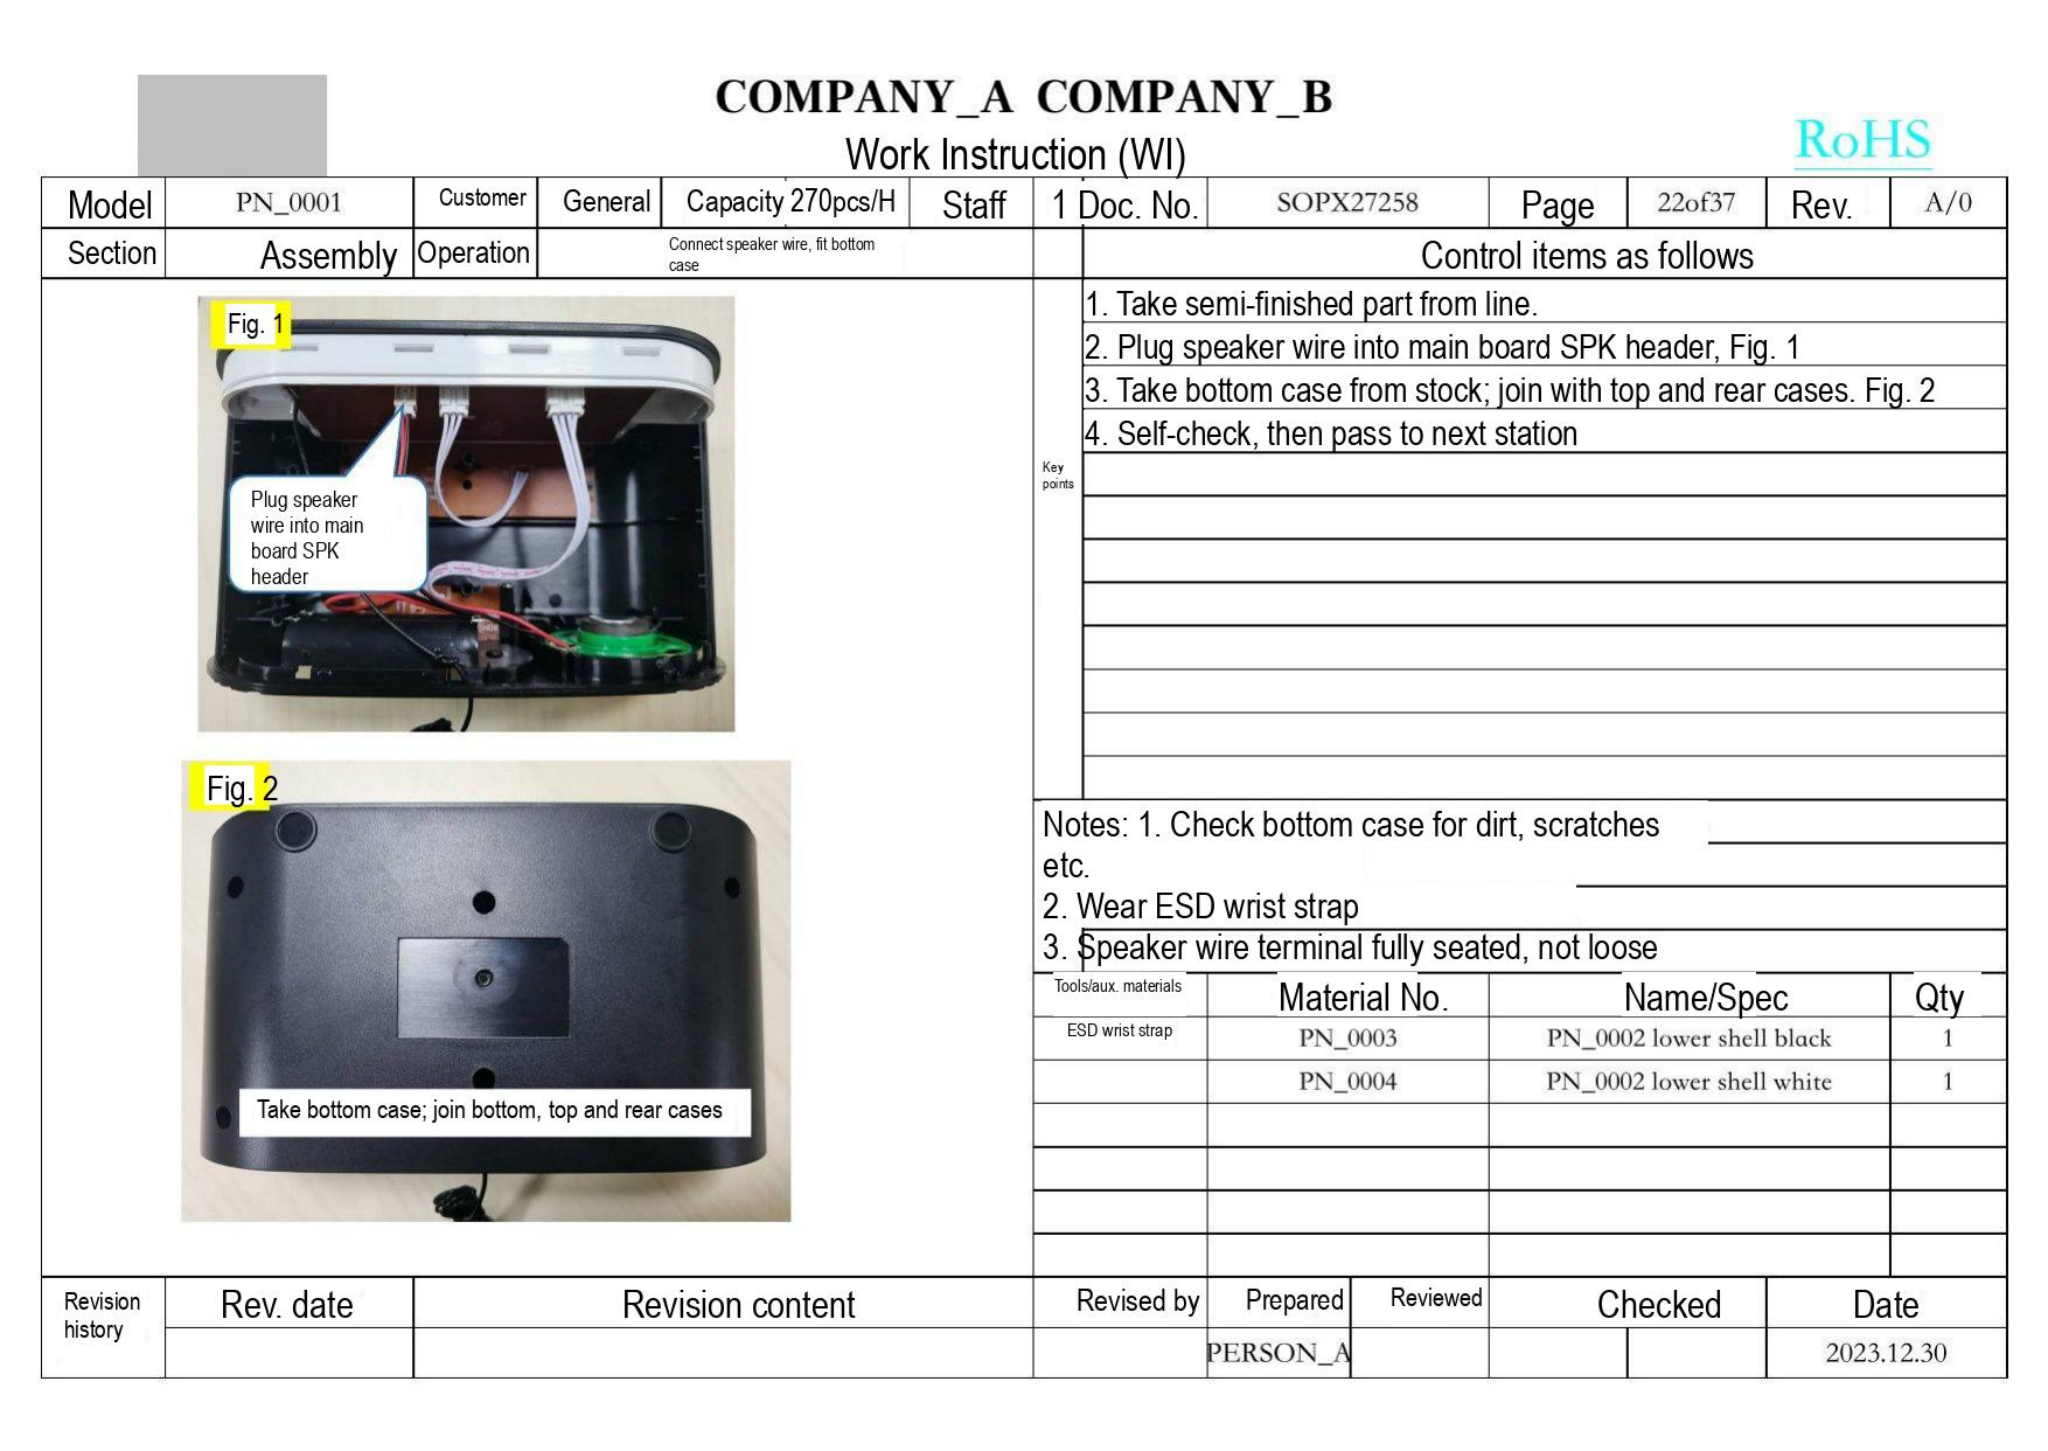COMPANY_A COMPANY_B
Work Instruction (WI)
RoHS

| Model | PN_0001 | Customer | General | Capacity 270pcs/H | Staff | 1 | Doc. No. | SOPX27258 | Page | 22of37 | Rev. | A/0 |
|---|---|---|---|---|---|---|---|---|---|---|---|---|
| Section | Assembly | Operation | Connect speaker wire, fit bottom case | | | | | | | | | |

Fig. 1
Plug speaker wire into main board SPK header

Fig. 2
Take bottom case; join bottom, top and rear cases

| Key points | Control items as follows |
|---|---|
| | 1. Take semi-finished part from line. |
| | 2. Plug speaker wire into main board SPK header, Fig. 1 |
| | 3. Take bottom case from stock; join with top and rear cases. Fig. 2 |
| | 4. Self-check, then pass to next station |

Notes: 1. Check bottom case for dirt, scratches etc.
2. Wear ESD wrist strap
3. Speaker wire terminal fully seated, not loose

| Tools/aux. materials | Material No. | Name/Spec | Qty |
|---|---|---|---|
| ESD wrist strap | PN_0003 | PN_0002 lower shell black | 1 |
| | PN_0004 | PN_0002 lower shell white | 1 |

| Revision history | Rev. date | Revision content | Revised by | Prepared | Reviewed | Checked | Date |
|---|---|---|---|---|---|---|---|
| | | | | PERSON_A | | | 2023.12.30 |
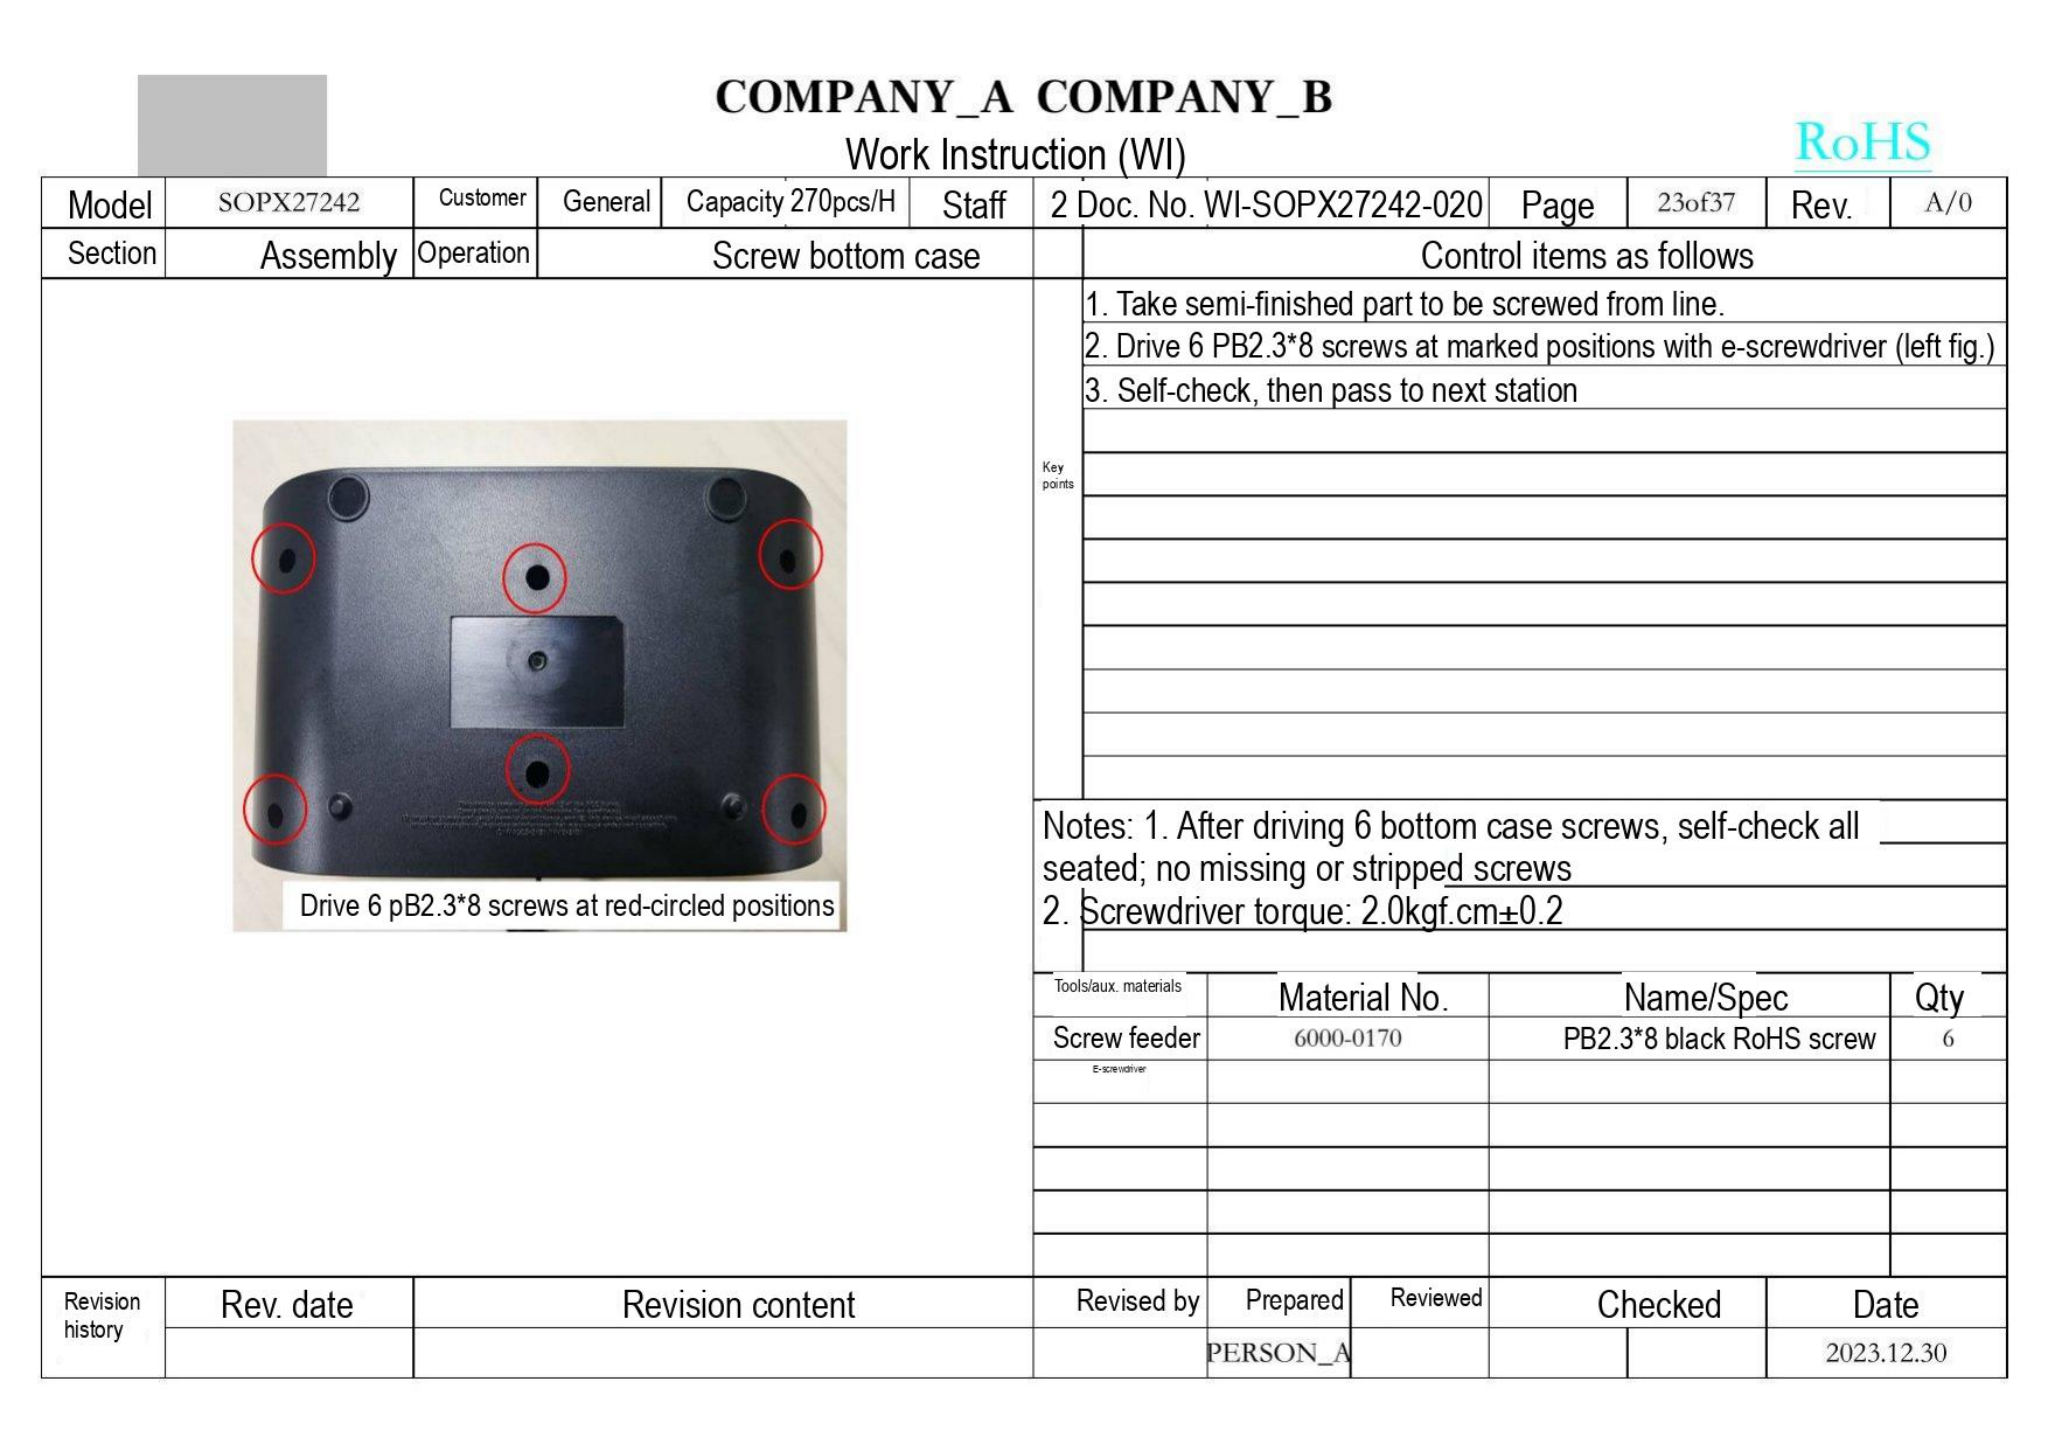COMPANY_A COMPANY_B
Work Instruction (WI)
RoHS

| Model | SOPX27242 | Customer | General | Capacity | 270pcs/H | Staff | 2 | Doc. No. | WI-SOPX27242-020 | Page | 23of37 | Rev. | A/0 |
|---|---|---|---|---|---|---|---|---|---|---|---|---|---|
| Section | Assembly | Operation | Screw bottom case | | | | | Control items as follows | | | | | |

Drive 6 pB2.3*8 screws at red-circled positions

Key points
1. Take semi-finished part to be screwed from line.
2. Drive 6 PB2.3*8 screws at marked positions with e-screwdriver (left fig.)
3. Self-check, then pass to next station

Notes: 1. After driving 6 bottom case screws, self-check all seated; no missing or stripped screws
2. Screwdriver torque: 2.0kgf.cm±0.2

| Tools/aux. materials | Material No. | Name/Spec | Qty |
|---|---|---|---|
| Screw feeder<br>E-screwdriver | 6000-0170 | PB2.3*8 black RoHS screw | 6 |
| | | | |
| | | | |
| | | | |
| | | | |
| | | | |

| Revision history | Rev. date | Revision content | Revised by | Prepared | Reviewed | Checked | Date |
|---|---|---|---|---|---|---|---|
| | | | | PERSON_A | | | 2023.12.30 |
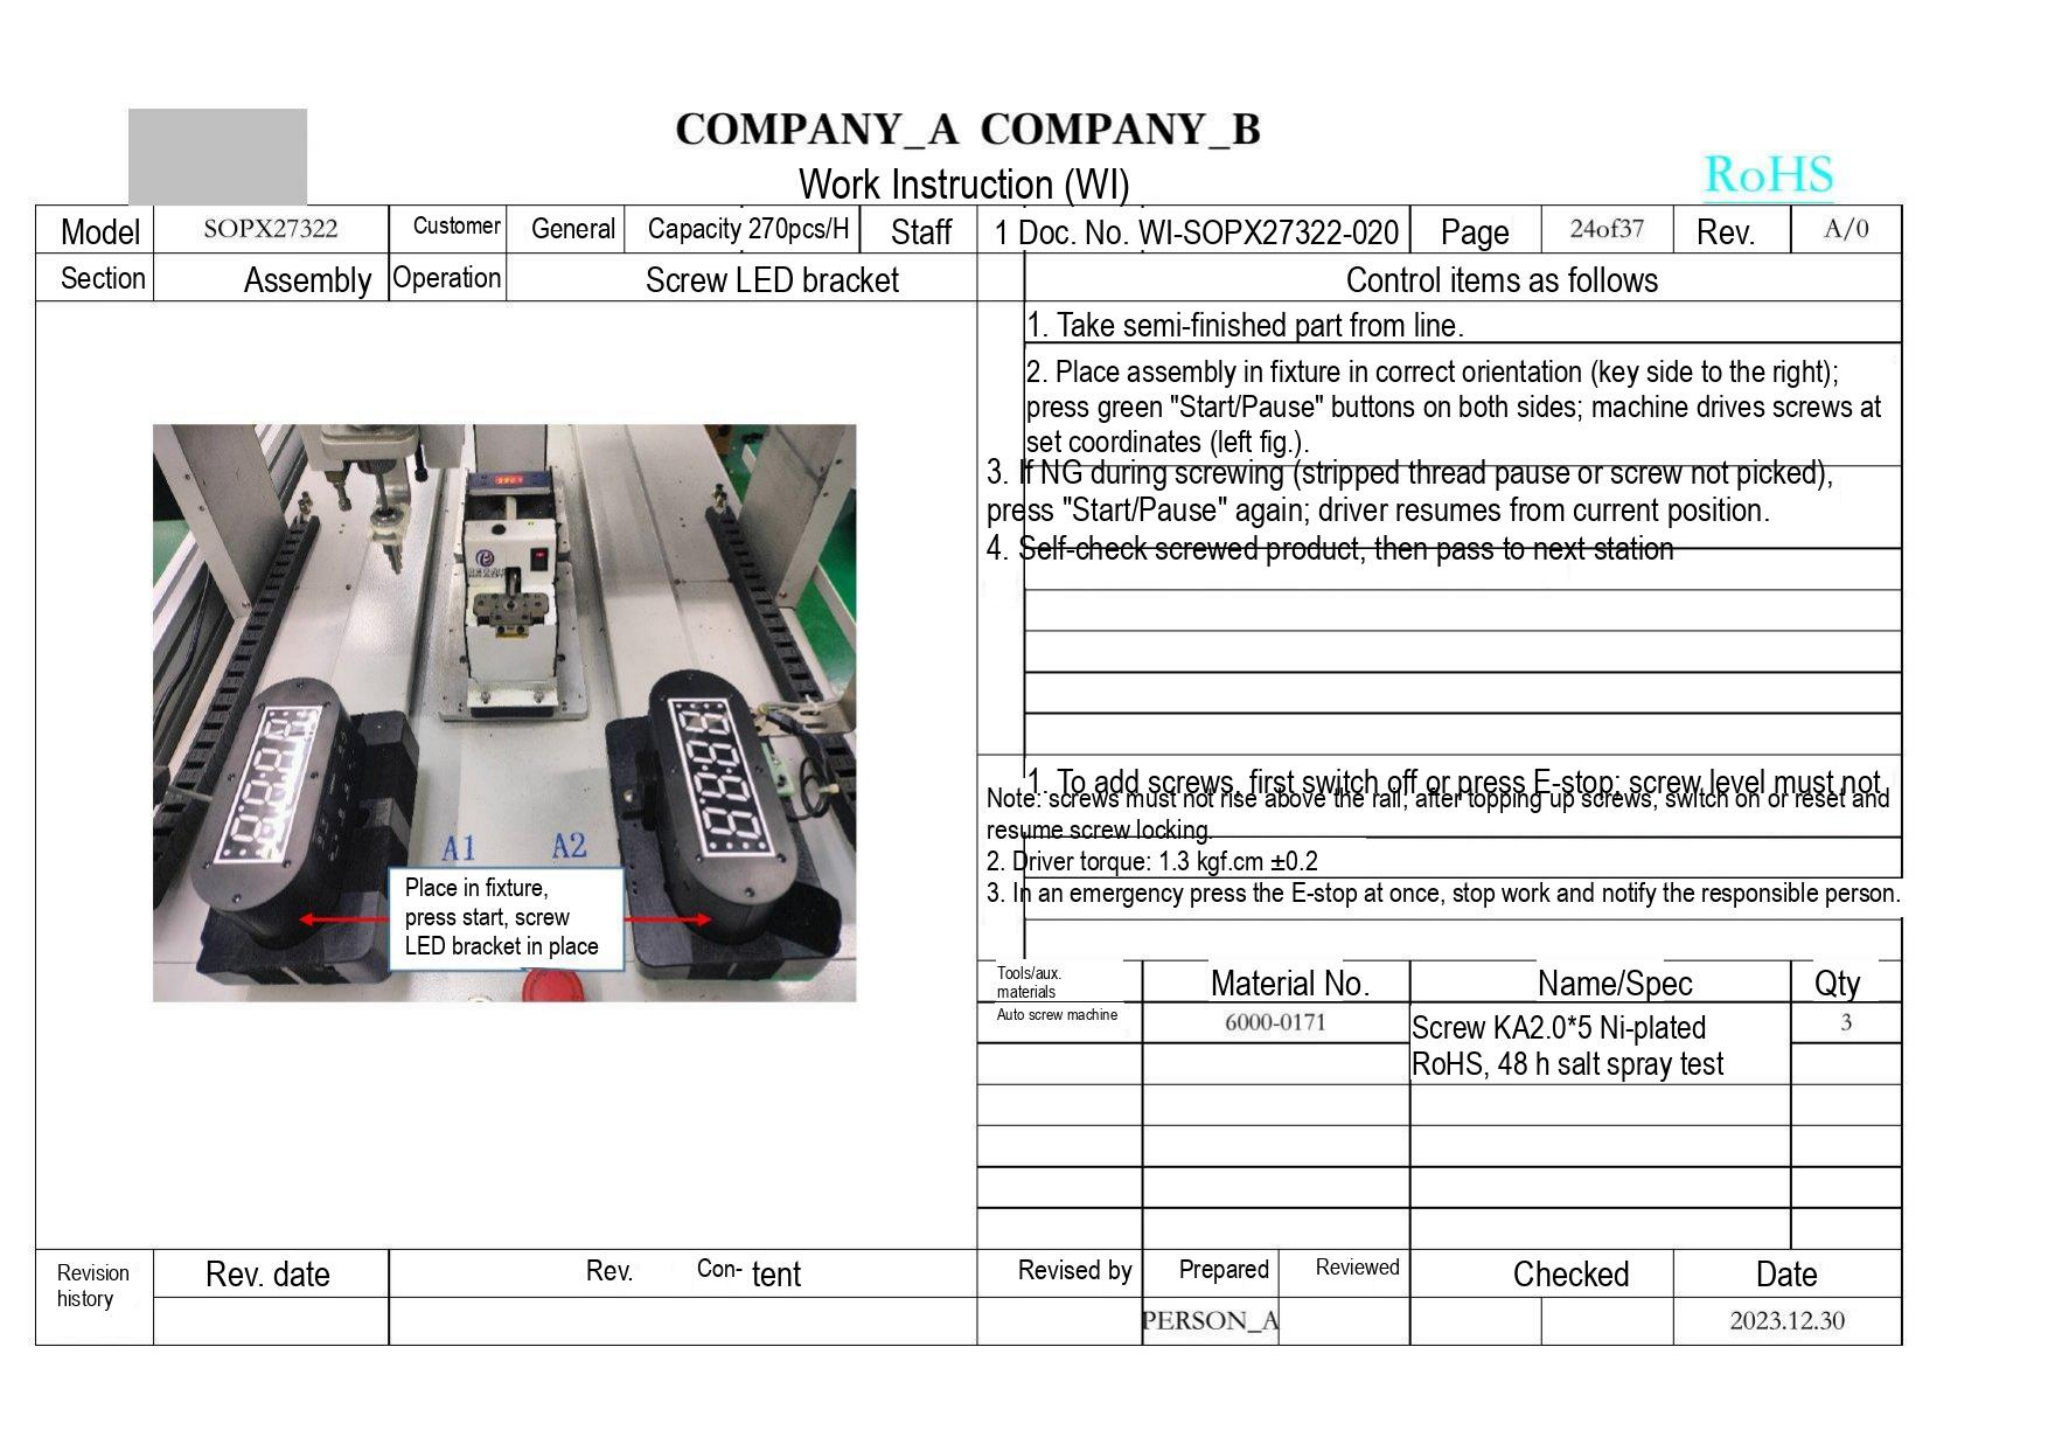# COMPANY_A COMPANY_B

Work Instruction (WI)

RoHS

| Model | SOPX27322 | Customer | General | Capacity 270pcs/H | Staff | 1 Doc. No. WI-SOPX27322-020 | Page | 24of37 | Rev. | A/0 |
|---|---|---|---|---|---|---|---|---|---|---|
| Section | Assembly | Operation | Screw LED bracket | | | | | | | |

A1 A2

Place in fixture, press start, screw LED bracket in place

Control items as follows

1. Take semi-finished part from line.
2. Place assembly in fixture in correct orientation (key side to the right); press green "Start/Pause" buttons on both sides; machine drives screws at set coordinates (left fig.).
3. If NG during screwing (stripped thread pause or screw not picked), press "Start/Pause" again; driver resumes from current position.
4. Self-check screwed product, then pass to next station

Note: 1. To add screws, first switch off or press E-stop; screw level must not
screws must not rise above the rail, after topping up screws, switch on or reset and resume screw locking.
2. Driver torque: 1.3 kgf.cm ±0.2
3. In an emergency press the E-stop at once, stop work and notify the responsible person.

| Tools/aux. materials | Material No. | Name/Spec | Qty |
|---|---|---|---|
| Auto screw machine | 6000-0171 | Screw KA2.0*5 Ni-plated RoHS, 48 h salt spray test | 3 |
| | | | |
| | | | |
| | | | |
| | | | |
| | | | |

| Revision history | Rev. date | Rev. Con- tent | Revised by | Prepared | Reviewed | Checked | Date |
|---|---|---|---|---|---|---|---|
| | | | | PERSON_A | | | 2023.12.30 |
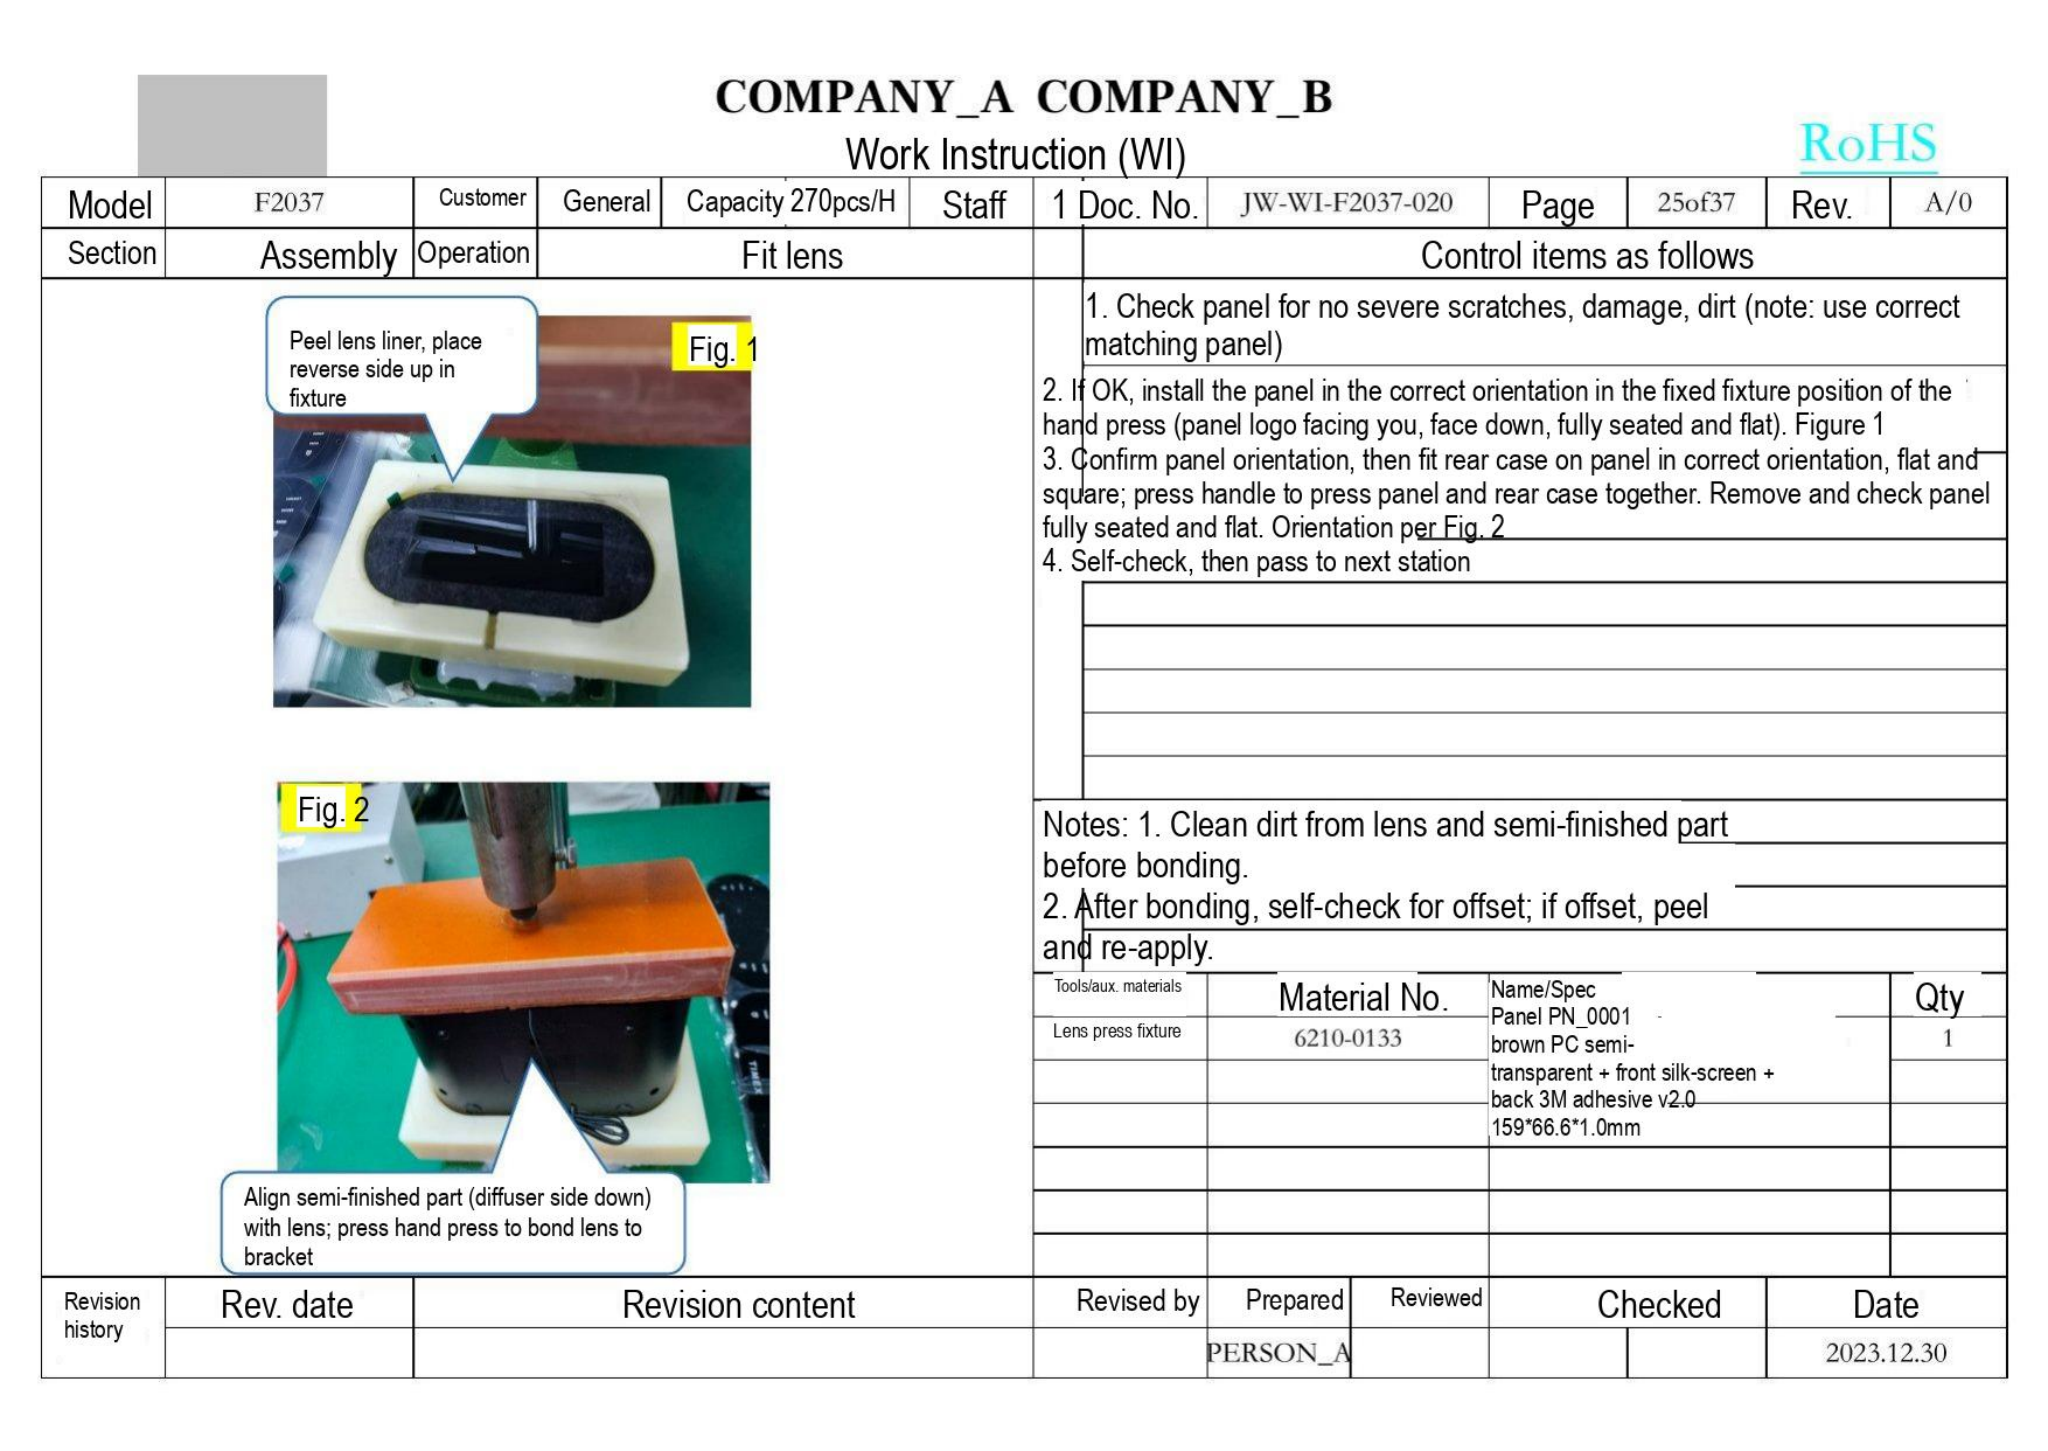COMPANY_A COMPANY_B
Work Instruction (WI)
RoHS

| Model | F2037 | Customer | General | Capacity 270pcs/H | Staff | 1 | Doc. No. | JW-WI-F2037-020 | Page | 25of37 | Rev. | A/0 |
|---|---|---|---|---|---|---|---|---|---|---|---|---|
| Section | Assembly | Operation | Fit lens | | | | | | | | | |

Peel lens liner, place reverse side up in fixture

Fig. 1

Fig. 2

Align semi-finished part (diffuser side down) with lens; press hand press to bond lens to bracket

Control items as follows

1. Check panel for no severe scratches, damage, dirt (note: use correct matching panel)
2. If OK, install the panel in the correct orientation in the fixed fixture position of the hand press (panel logo facing you, face down, fully seated and flat). Figure 1
3. Confirm panel orientation, then fit rear case on panel in correct orientation, flat and square; press handle to press panel and rear case together. Remove and check panel fully seated and flat. Orientation per Fig. 2
4. Self-check, then pass to next station

Notes: 1. Clean dirt from lens and semi-finished part before bonding.
2. After bonding, self-check for offset; if offset, peel and re-apply.

| Tools/aux. materials | Material No. | Name/Spec | Qty |
|---|---|---|---|
| Lens press fixture | 6210-0133 | Panel PN_0001 brown PC semi-transparent + front silk-screen + back 3M adhesive v2.0 159*66.6*1.0mm | 1 |
| | | | |
| | | | |
| | | | |
| | | | |
| | | | |

| Revision history | Rev. date | Revision content | Revised by | Prepared | Reviewed | Checked | Date |
|---|---|---|---|---|---|---|---|
| | | | | PERSON_A | | | 2023.12.30 |
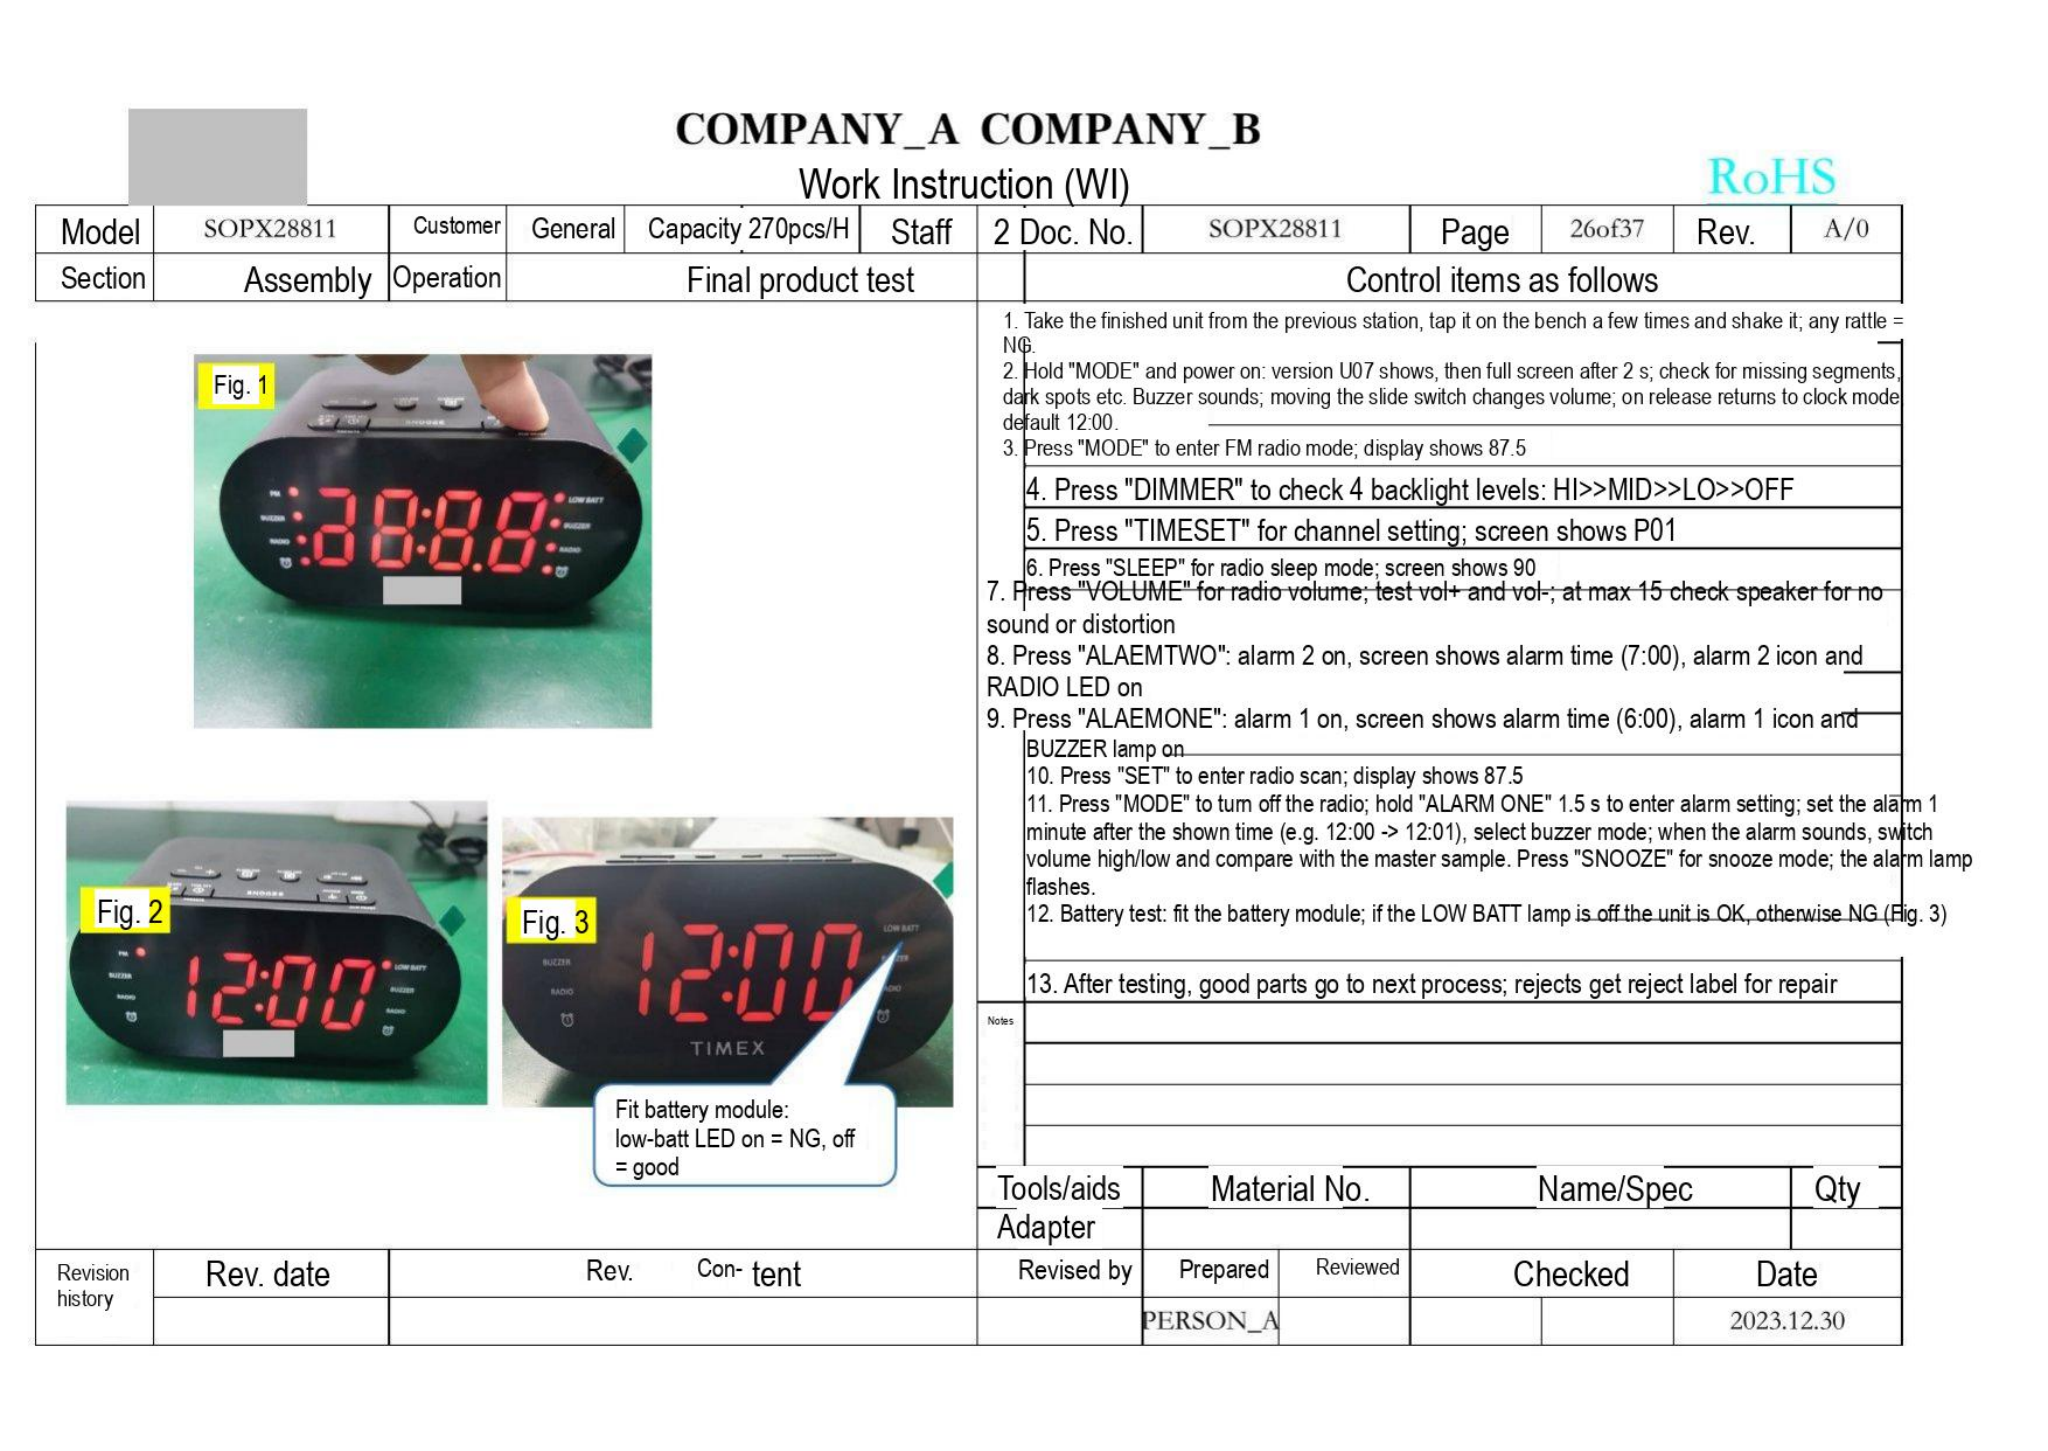COMPANY_A COMPANY_B
Work Instruction (WI)
RoHS

| Model | SOPX28811 | Customer | General | Capacity 270pcs/H | Staff | 2 Doc. No. | SOPX28811 | Page | 26of37 | Rev. | A/0 |
|---|---|---|---|---|---|---|---|---|---|---|---|
| Section | Assembly | Operation | Final product test | | | Control items as follows | | | | | |

Fig. 1
LOW BATT
BUZZER
RADIO
SNOOZE

Fig. 2
12:00
LOW BATT
BUZZER
RADIO
SNOOZE

Fig. 3
12:00
LOW BATT
BUZZER
RADIO
TIMEX

Fit battery module:
low-batt LED on = NG, off = good

1. Take the finished unit from the previous station, tap it on the bench a few times and shake it; any rattle = NG.
2. Hold "MODE" and power on: version U07 shows, then full screen after 2 s; check for missing segments, dark spots etc. Buzzer sounds; moving the slide switch changes volume; on release returns to clock mode default 12:00.
3. Press "MODE" to enter FM radio mode; display shows 87.5
4. Press "DIMMER" to check 4 backlight levels: HI>>MID>>LO>>OFF
5. Press "TIMESET" for channel setting; screen shows P01
6. Press "SLEEP" for radio sleep mode; screen shows 90
7. Press "VOLUME" for radio volume; test vol+ and vol-; at max 15 check speaker for no sound or distortion
8. Press "ALAEMTWO": alarm 2 on, screen shows alarm time (7:00), alarm 2 icon and RADIO LED on
9. Press "ALAEMONE": alarm 1 on, screen shows alarm time (6:00), alarm 1 icon and BUZZER lamp on
10. Press "SET" to enter radio scan; display shows 87.5
11. Press "MODE" to turn off the radio; hold "ALARM ONE" 1.5 s to enter alarm setting; set the alarm 1 minute after the shown time (e.g. 12:00 -> 12:01), select buzzer mode; when the alarm sounds, switch volume high/low and compare with the master sample. Press "SNOOZE" for snooze mode; the alarm lamp flashes.
12. Battery test: fit the battery module; if the LOW BATT lamp is off the unit is OK, otherwise NG (Fig. 3)
13. After testing, good parts go to next process; rejects get reject label for repair

Notes

| Tools/aids | Material No. | Name/Spec | Qty |
|---|---|---|---|
| Adapter | | | |

| Revision history | Rev. date | Rev. Con- tent | Revised by | Prepared | Reviewed | Checked | Date |
|---|---|---|---|---|---|---|---|
| | | | | PERSON_A | | | 2023.12.30 |
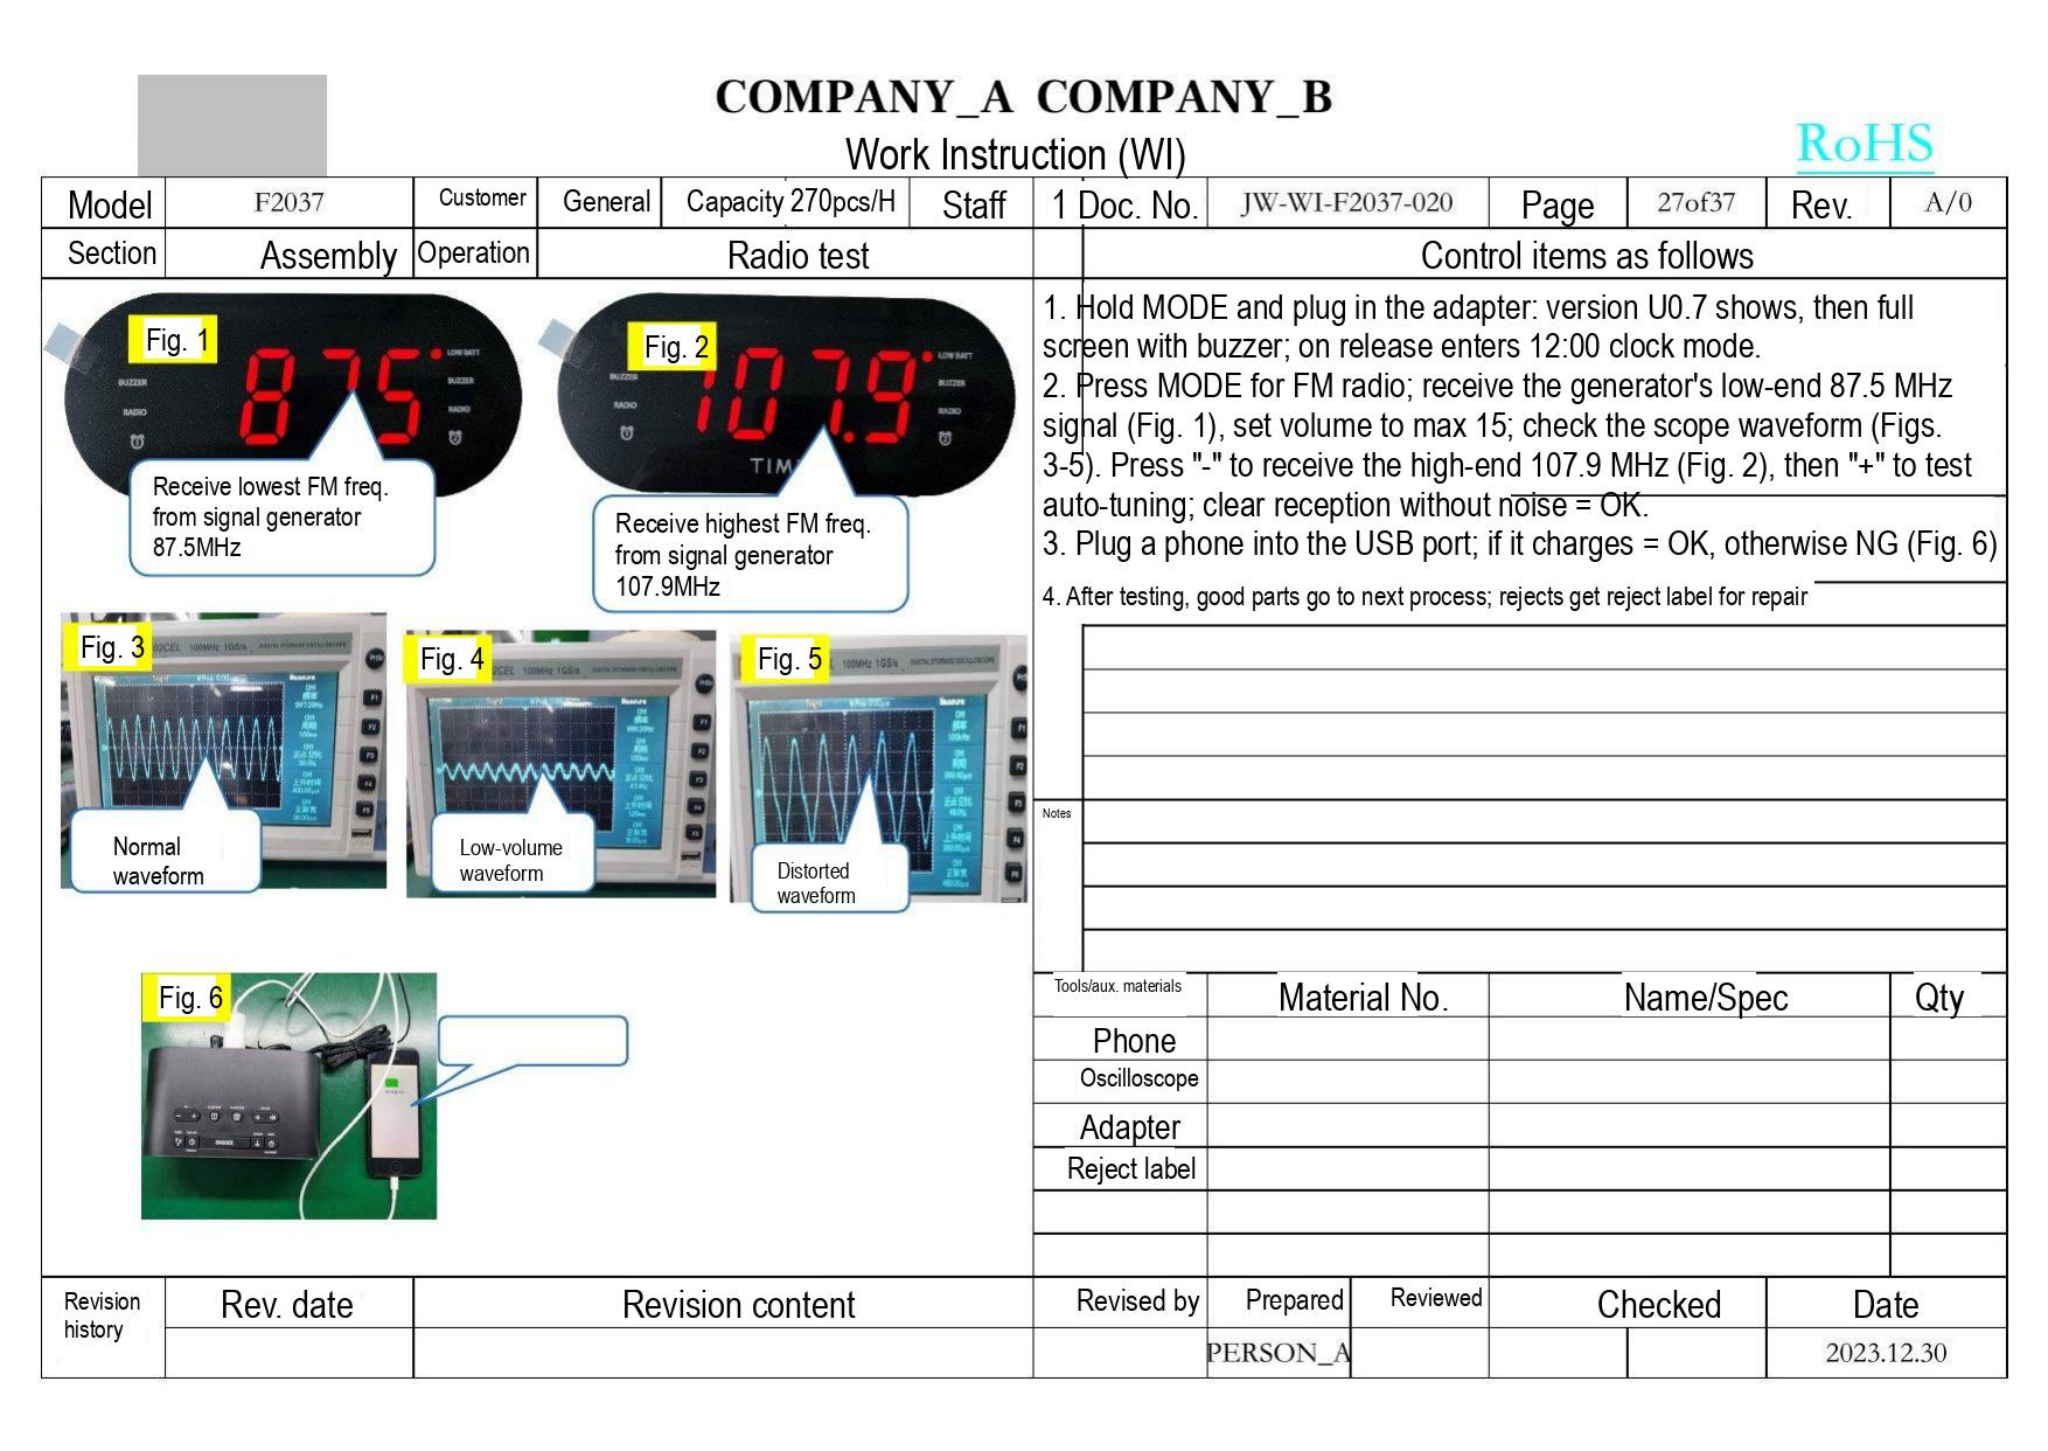COMPANY_A COMPANY_B
Work Instruction (WI)
RoHS

| Model | F2037 | Customer | General | Capacity 270pcs/H | Staff | 1 Doc. No. | JW-WI-F2037-020 | Page | 27of37 | Rev. | A/0 |
|---|---|---|---|---|---|---|---|---|---|---|---|
| Section | Assembly | Operation | Radio test | | | Control items as follows | | | | | |

Fig. 1
875
Receive lowest FM freq. from signal generator 87.5MHz

Fig. 2
107.9
Receive highest FM freq. from signal generator 107.9MHz

Fig. 3
Normal waveform

Fig. 4
Low-volume waveform

Fig. 5
Distorted waveform

Fig. 6

Control items as follows

1. Hold MODE and plug in the adapter: version U0.7 shows, then full screen with buzzer; on release enters 12:00 clock mode.
2. Press MODE for FM radio; receive the generator's low-end 87.5 MHz signal (Fig. 1), set volume to max 15; check the scope waveform (Figs. 3-5). Press "-" to receive the high-end 107.9 MHz (Fig. 2), then "+" to test auto-tuning; clear reception without noise = OK.
3. Plug a phone into the USB port; if it charges = OK, otherwise NG (Fig. 6)
4. After testing, good parts go to next process; rejects get reject label for repair

Notes

| Tools/aux. materials | Material No. | Name/Spec | Qty |
|---|---|---|---|
| Phone | | | |
| Oscilloscope | | | |
| Adapter | | | |
| Reject label | | | |
| | | | |
| | | | |

| Revision history | Rev. date | Revision content | Revised by | Prepared | Reviewed | Checked | Date |
|---|---|---|---|---|---|---|---|
| | | | | PERSON_A | | | 2023.12.30 |
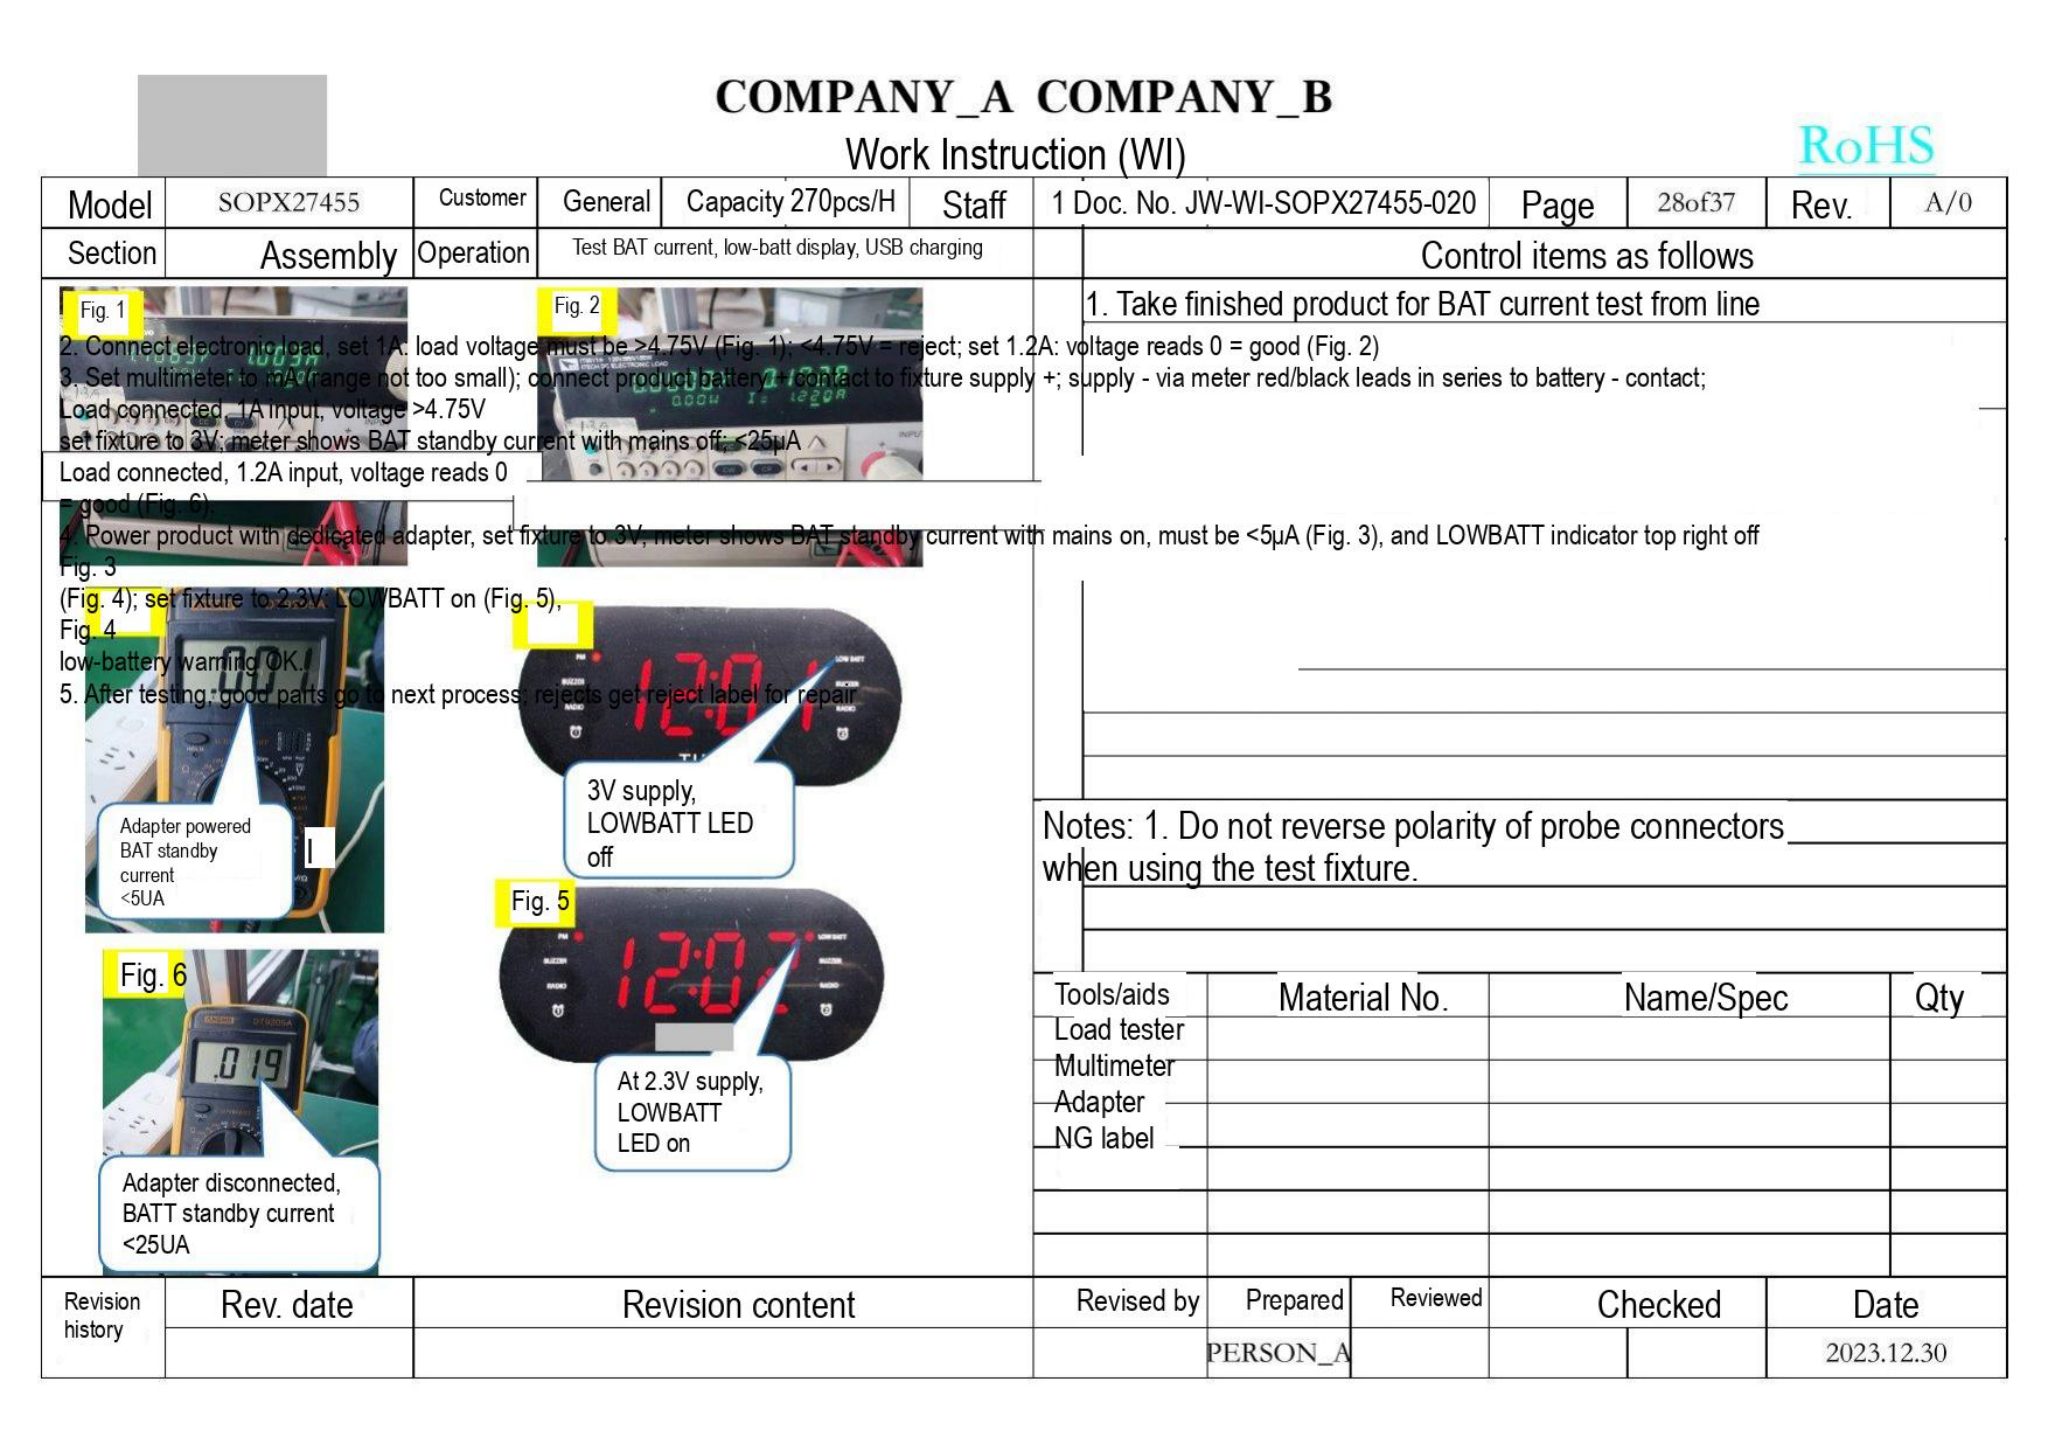COMPANY_A COMPANY_B

Work Instruction (WI)

RoHS

| Model | SOPX27455 | Customer | General | Capacity 270pcs/H | Staff | 1 Doc. No. JW-WI-SOPX27455-020 | Page | 28of37 | Rev. | A/0 |
|---|---|---|---|---|---|---|---|---|---|---|
| Section | Assembly | Operation | Test BAT current, low-batt display, USB charging | | | Control items as follows | | | | |

1. Take finished product for BAT current test from line

Fig. 1

Fig. 2

2. Connect electronic load, set 1A: load voltage must be >4.75V (Fig. 1); <4.75V = reject; set 1.2A: voltage reads 0 = good (Fig. 2)

3. Set multimeter to mA (range not too small); connect product battery + contact to fixture supply +; supply - via meter red/black leads in series to battery - contact;

Load connected, 1A input, voltage >4.75V

set fixture to 3V; meter shows BAT standby current with mains off; <25μA

Load connected, 1.2A input, voltage reads 0

= good (Fig. 6).

4. Power product with dedicated adapter, set fixture to 3V; meter shows BAT standby current with mains on, must be <5μA (Fig. 3), and LOWBATT indicator top right off

Fig. 3

(Fig. 4); set fixture to 2.3V: LOWBATT on (Fig. 5),

Fig. 4

low-battery warning OK.

5. After testing, good parts go to next process; rejects get reject label for repair

Adapter powered BAT standby current <5UA

3V supply, LOWBATT LED off

Fig. 5

At 2.3V supply, LOWBATT LED on

Fig. 6

Adapter disconnected, BATT standby current <25UA

Notes: 1. Do not reverse polarity of probe connectors when using the test fixture.

| Tools/aids | Material No. | Name/Spec | Qty |
|---|---|---|---|
| Load tester | | | |
| Multimeter | | | |
| Adapter | | | |
| NG label | | | |

| Revision history | Rev. date | Revision content | Revised by | Prepared | Reviewed | Checked | Date |
|---|---|---|---|---|---|---|---|
| | | | | PERSON_A | | | 2023.12.30 |